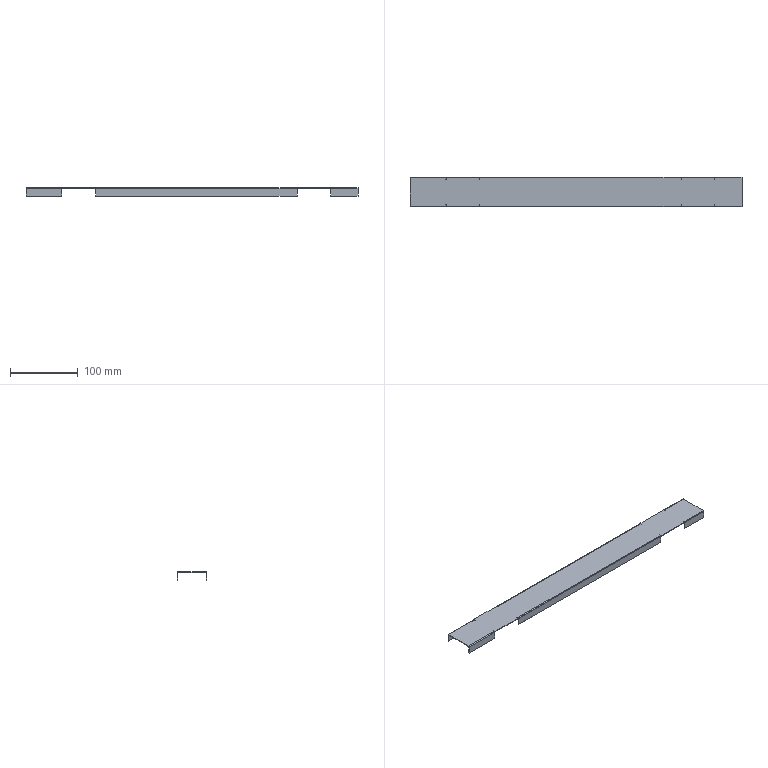Part | 1 solid | 86 faces | box 490 x 44 x 12 mm | volume 29894 mm3 | plane 74 | cylinder 12 | commonest cylinder face diameters 0.4 x6 2.4 x6